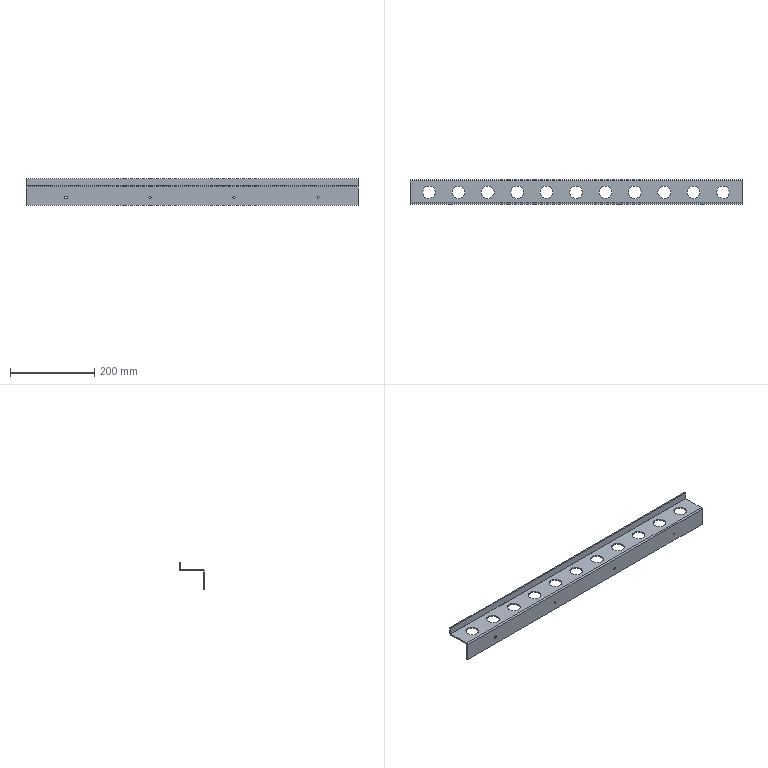Part | STEP file | HESS-408-70-15W-W-7-outer case reinforcing rib 3 | 1 solid | 44 faces | box 790 x 58.5 x 64 mm | volume 256348 mm3 | cylinder 34 | plane 10 | commonest cylinder face diameters 30 x22 5 x6 0.2 x2 6.2 x2 6.8 x2